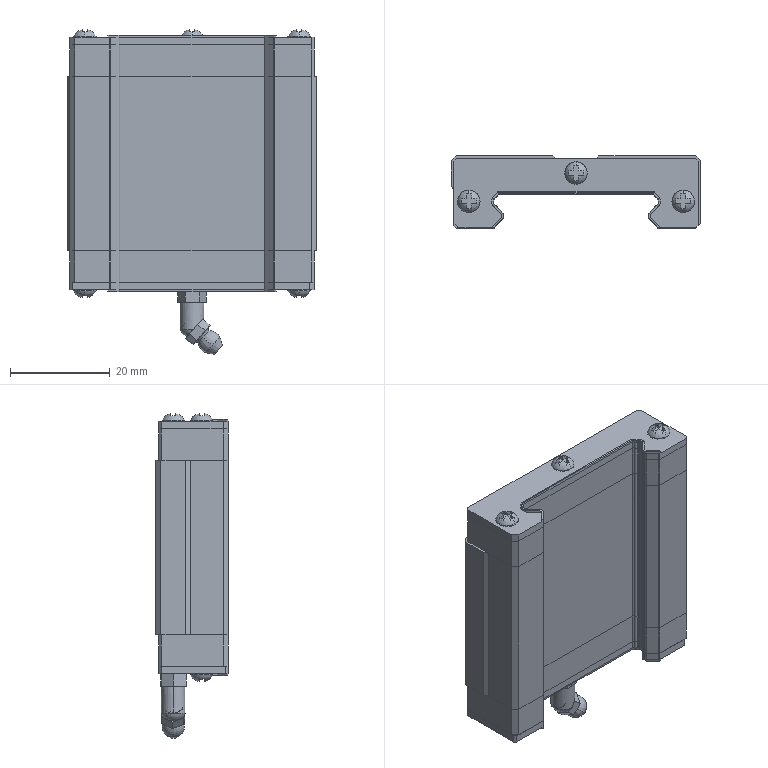Part | SolidWorks | 12 solids | 577 faces | box 50 x 14.5 x 65.112 mm | volume 24811 mm3 | plane 311 | cylinder 149 | cone 74 | spline 22 | torus 21 | commonest cylinder face diameters 1 x50 0.77 x30 3 x26 4 x13 4.5 x12 3.3 x10